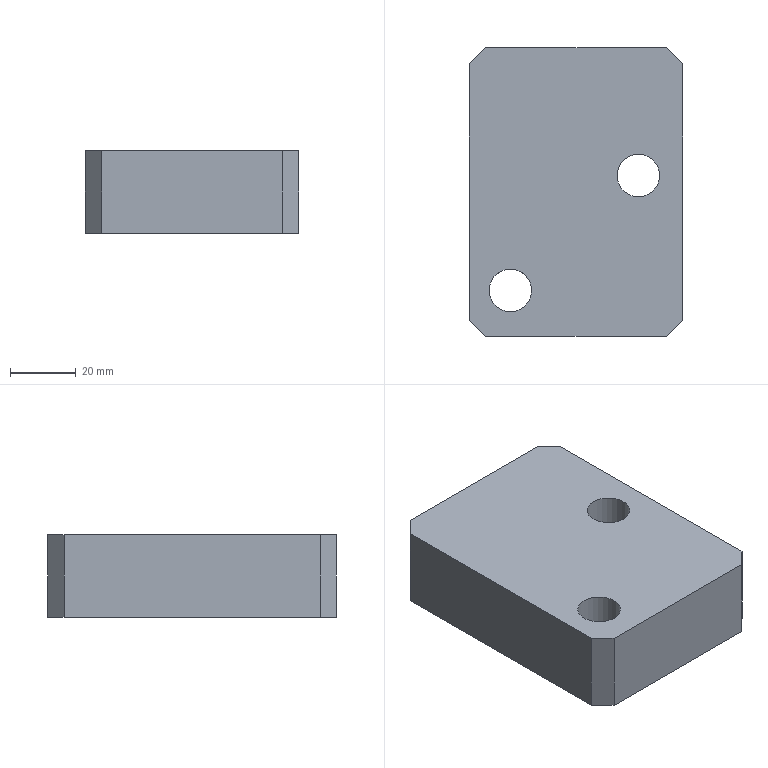Part | STEP file | 433_id2094_x_t | 1 solid | 16 faces | box 65 x 88 x 25 mm | volume 129688 mm3 | plane 12 | cylinder 4 | commonest cylinder face diameters 13 x2 20 x2
STEP:
#1=CARTESIAN_POINT('',(0.,0.,0.));
#2=DIRECTION('',(0.,0.,1.));
#3=DIRECTION('',(1.,0.,0.));
#4=AXIS2_PLACEMENT_3D('',#1,#2,#3);
#5=CARTESIAN_POINT('',(-51.,-323.071,3.));
#6=VERTEX_POINT('',#5);
#7=CARTESIAN_POINT('',(-51.,-245.,3.));
#8=VERTEX_POINT('',#7);
#9=CARTESIAN_POINT('',(-51.,625.206,3.));
#10=DIRECTION('',(0.,1.,0.));
#11=VECTOR('',#10,1.);
#12=LINE('',#9,#11);
#13=CARTESIAN_POINT('',(-51.,617.983,-1.));
#14=DIRECTION('',(-1.,0.,0.));
#15=DIRECTION('',(0.,0.,1.));
#16=AXIS2_PLACEMENT_3D('',#13,#14,#15);
#17=PLANE('',#16);
#18=CARTESIAN_POINT('',(4.,7.223));
#19=DIRECTION('',(0.,1.));
#20=VECTOR('',#19,1.);
#21=LINE('',#18,#20);
#22=(GEOMETRIC_REPRESENTATION_CONTEXT(2)PARAMETRIC_REPRESENTATION_CONTEXT()REPRESENTATION_CONTEXT('',''));
#23=DEFINITIONAL_REPRESENTATION('',(#21),#22);
#24=PCURVE('',#17,#23);
#25=CARTESIAN_POINT('',(-678.966,625.206,3.));
#26=DIRECTION('',(0.,0.,1.));
#27=DIRECTION('',(1.,0.,0.));
#28=AXIS2_PLACEMENT_3D('',#25,#26,#27);
#29=PLANE('',#28);
#30=CARTESIAN_POINT('',(627.966,0.));
#31=DIRECTION('',(0.,1.));
#32=VECTOR('',#31,1.);
#33=LINE('',#30,#32);
#34=(GEOMETRIC_REPRESENTATION_CONTEXT(2)PARAMETRIC_REPRESENTATION_CONTEXT()REPRESENTATION_CONTEXT('',''));
#35=DEFINITIONAL_REPRESENTATION('',(#33),#34);
#36=PCURVE('',#29,#35);
#37=SURFACE_CURVE('',#12,(#24,#36),.PCURVE_S1.);
#38=EDGE_CURVE('',#6,#8,#37,.T.);
#39=ORIENTED_EDGE('',*,*,#38,.T.);
#40=CARTESIAN_POINT('',(-51.,-245.,-22.));
#41=VERTEX_POINT('',#40);
#42=CARTESIAN_POINT('',(-51.,-245.,-17.));
#43=DIRECTION('',(0.,0.,1.));
#44=VECTOR('',#43,1.);
#45=LINE('',#42,#44);
#46=CARTESIAN_POINT('',(-16.,-862.983));
#47=DIRECTION('',(1.,0.));
#48=VECTOR('',#47,1.);
#49=LINE('',#46,#48);
#50=(GEOMETRIC_REPRESENTATION_CONTEXT(2)PARAMETRIC_REPRESENTATION_CONTEXT()REPRESENTATION_CONTEXT('',''));
#51=DEFINITIONAL_REPRESENTATION('',(#49),#50);
#52=PCURVE('',#17,#51);
#53=CARTESIAN_POINT('',(-51.,-245.,-1.));
#54=DIRECTION('',(0.7071,-0.7071,0.));
#55=DIRECTION('',(0.,0.,1.));
#56=AXIS2_PLACEMENT_3D('',#53,#54,#55);
#57=PLANE('',#56);
#58=CARTESIAN_POINT('',(-16.,0.));
#59=DIRECTION('',(1.,0.));
#60=VECTOR('',#59,1.);
#61=LINE('',#58,#60);
#62=(GEOMETRIC_REPRESENTATION_CONTEXT(2)PARAMETRIC_REPRESENTATION_CONTEXT()REPRESENTATION_CONTEXT('',''));
#63=DEFINITIONAL_REPRESENTATION('',(#61),#62);
#64=PCURVE('',#57,#63);
#65=SURFACE_CURVE('',#45,(#52,#64),.PCURVE_S1.);
#66=EDGE_CURVE('',#41,#8,#65,.T.);
#67=ORIENTED_EDGE('',*,*,#66,.F.);
#68=CARTESIAN_POINT('',(-51.,-323.071,-22.));
#69=VERTEX_POINT('',#68);
#70=CARTESIAN_POINT('',(-51.,625.206,-22.));
#71=DIRECTION('',(0.,1.,0.));
#72=VECTOR('',#71,1.);
#73=LINE('',#70,#72);
#74=CARTESIAN_POINT('',(-21.,7.223));
#75=DIRECTION('',(0.,1.));
#76=VECTOR('',#75,1.);
#77=LINE('',#74,#76);
#78=(GEOMETRIC_REPRESENTATION_CONTEXT(2)PARAMETRIC_REPRESENTATION_CONTEXT()REPRESENTATION_CONTEXT('',''));
#79=DEFINITIONAL_REPRESENTATION('',(#77),#78);
#80=PCURVE('',#17,#79);
#81=CARTESIAN_POINT('',(-678.966,625.206,-22.));
#82=DIRECTION('',(0.,0.,1.));
#83=DIRECTION('',(1.,0.,0.));
#84=AXIS2_PLACEMENT_3D('',#81,#82,#83);
#85=PLANE('',#84);
#86=CARTESIAN_POINT('',(627.966,0.));
#87=DIRECTION('',(0.,1.));
#88=VECTOR('',#87,1.);
#89=LINE('',#86,#88);
#90=(GEOMETRIC_REPRESENTATION_CONTEXT(2)PARAMETRIC_REPRESENTATION_CONTEXT()REPRESENTATION_CONTEXT('',''));
#91=DEFINITIONAL_REPRESENTATION('',(#89),#90);
#92=PCURVE('',#85,#91);
#93=SURFACE_CURVE('',#73,(#80,#92),.PCURVE_S1.);
#94=EDGE_CURVE('',#69,#41,#93,.T.);
#95=ORIENTED_EDGE('',*,*,#94,.F.);
#96=CARTESIAN_POINT('',(-51.,-323.071,-1.));
#97=DIRECTION('',(0.,0.,-1.));
#98=VECTOR('',#97,1.);
#99=LINE('',#96,#98);
#100=CARTESIAN_POINT('',(0.,-941.054));
#101=DIRECTION('',(-1.,0.));
#102=VECTOR('',#101,1.);
#103=LINE('',#100,#102);
#104=(GEOMETRIC_REPRESENTATION_CONTEXT(2)PARAMETRIC_REPRESENTATION_CONTEXT()REPRESENTATION_CONTEXT('',''));
#105=DEFINITIONAL_REPRESENTATION('',(#103),#104);
#106=PCURVE('',#17,#105);
#107=CARTESIAN_POINT('',(-47.536,-326.536,49.));
#108=DIRECTION('',(0.7071,0.7071,0.));
#109=DIRECTION('',(0.,0.,1.));
#110=AXIS2_PLACEMENT_3D('',#107,#108,#109);
#111=PLANE('',#110);
#112=CARTESIAN_POINT('',(-50.,-4.899));
#113=DIRECTION('',(-1.,0.));
#114=VECTOR('',#113,1.);
#115=LINE('',#112,#114);
#116=(GEOMETRIC_REPRESENTATION_CONTEXT(2)PARAMETRIC_REPRESENTATION_CONTEXT()REPRESENTATION_CONTEXT('',''));
#117=DEFINITIONAL_REPRESENTATION('',(#115),#116);
#118=PCURVE('',#111,#117);
#119=SURFACE_CURVE('',#99,(#106,#118),.PCURVE_S1.);
#120=EDGE_CURVE('',#6,#69,#119,.T.);
#121=ORIENTED_EDGE('',*,*,#120,.F.);
#122=EDGE_LOOP('',(#39,#67,#95,#121));
#123=FACE_BOUND('',#122,.T.);
#124=ADVANCED_FACE('',(#123),#17,.T.);
#125=CARTESIAN_POINT('',(14.,-245.,-22.));
#126=VERTEX_POINT('',#125);
#127=CARTESIAN_POINT('',(14.,-323.071,-22.));
#128=VERTEX_POINT('',#127);
#129=CARTESIAN_POINT('',(14.,625.206,-22.));
#130=DIRECTION('',(0.,-1.,0.));
#131=VECTOR('',#130,1.);
#132=LINE('',#129,#131);
#133=CARTESIAN_POINT('',(14.,617.983,-1.));
#134=DIRECTION('',(1.,0.,0.));
#135=DIRECTION('',(0.,0.,-1.));
#136=AXIS2_PLACEMENT_3D('',#133,#134,#135);
#137=PLANE('',#136);
#138=CARTESIAN_POINT('',(21.,7.223));
#139=DIRECTION('',(0.,-1.));
#140=VECTOR('',#139,1.);
#141=LINE('',#138,#140);
#142=(GEOMETRIC_REPRESENTATION_CONTEXT(2)PARAMETRIC_REPRESENTATION_CONTEXT()REPRESENTATION_CONTEXT('',''));
#143=DEFINITIONAL_REPRESENTATION('',(#141),#142);
#144=PCURVE('',#137,#143);
#145=CARTESIAN_POINT('',(692.966,0.));
#146=DIRECTION('',(0.,-1.));
#147=VECTOR('',#146,1.);
#148=LINE('',#145,#147);
#149=(GEOMETRIC_REPRESENTATION_CONTEXT(2)PARAMETRIC_REPRESENTATION_CONTEXT()REPRESENTATION_CONTEXT('',''));
#150=DEFINITIONAL_REPRESENTATION('',(#148),#149);
#151=PCURVE('',#85,#150);
#152=SURFACE_CURVE('',#132,(#144,#151),.PCURVE_S1.);
#153=EDGE_CURVE('',#126,#128,#152,.T.);
#154=ORIENTED_EDGE('',*,*,#153,.F.);
#155=CARTESIAN_POINT('',(14.,-245.,3.));
#156=VERTEX_POINT('',#155);
#157=CARTESIAN_POINT('',(14.,-245.,3.));
#158=DIRECTION('',(0.,0.,-1.));
#159=VECTOR('',#158,1.);
#160=LINE('',#157,#159);
#161=CARTESIAN_POINT('',(-4.,-862.983));
#162=DIRECTION('',(1.,0.));
#163=VECTOR('',#162,1.);
#164=LINE('',#161,#163);
#165=(GEOMETRIC_REPRESENTATION_CONTEXT(2)PARAMETRIC_REPRESENTATION_CONTEXT()REPRESENTATION_CONTEXT('',''));
#166=DEFINITIONAL_REPRESENTATION('',(#164),#165);
#167=PCURVE('',#137,#166);
#168=CARTESIAN_POINT('',(9.,-240.,4.));
#169=DIRECTION('',(-0.7071,-0.7071,0.));
#170=DIRECTION('',(0.,0.,1.));
#171=AXIS2_PLACEMENT_3D('',#168,#169,#170);
#172=PLANE('',#171);
#173=CARTESIAN_POINT('',(-1.,-7.071));
#174=DIRECTION('',(-1.,0.));
#175=VECTOR('',#174,1.);
#176=LINE('',#173,#175);
#177=(GEOMETRIC_REPRESENTATION_CONTEXT(2)PARAMETRIC_REPRESENTATION_CONTEXT()REPRESENTATION_CONTEXT('',''));
#178=DEFINITIONAL_REPRESENTATION('',(#176),#177);
#179=PCURVE('',#172,#178);
#180=SURFACE_CURVE('',#160,(#167,#179),.PCURVE_S1.);
#181=EDGE_CURVE('',#156,#126,#180,.T.);
#182=ORIENTED_EDGE('',*,*,#181,.F.);
#183=CARTESIAN_POINT('',(14.,-323.071,3.));
#184=VERTEX_POINT('',#183);
#185=CARTESIAN_POINT('',(14.,625.206,3.));
#186=DIRECTION('',(0.,-1.,0.));
#187=VECTOR('',#186,1.);
#188=LINE('',#185,#187);
#189=CARTESIAN_POINT('',(-4.,7.223));
#190=DIRECTION('',(0.,-1.));
#191=VECTOR('',#190,1.);
#192=LINE('',#189,#191);
#193=(GEOMETRIC_REPRESENTATION_CONTEXT(2)PARAMETRIC_REPRESENTATION_CONTEXT()REPRESENTATION_CONTEXT('',''));
#194=DEFINITIONAL_REPRESENTATION('',(#192),#193);
#195=PCURVE('',#137,#194);
#196=CARTESIAN_POINT('',(692.966,0.));
#197=DIRECTION('',(0.,-1.));
#198=VECTOR('',#197,1.);
#199=LINE('',#196,#198);
#200=(GEOMETRIC_REPRESENTATION_CONTEXT(2)PARAMETRIC_REPRESENTATION_CONTEXT()REPRESENTATION_CONTEXT('',''));
#201=DEFINITIONAL_REPRESENTATION('',(#199),#200);
#202=PCURVE('',#29,#201);
#203=SURFACE_CURVE('',#188,(#195,#202),.PCURVE_S1.);
#204=EDGE_CURVE('',#156,#184,#203,.T.);
#205=ORIENTED_EDGE('',*,*,#204,.T.);
#206=CARTESIAN_POINT('',(14.,-323.071,-1.));
#207=DIRECTION('',(0.,0.,1.));
#208=VECTOR('',#207,1.);
#209=LINE('',#206,#208);
#210=CARTESIAN_POINT('',(0.,-941.054));
#211=DIRECTION('',(-1.,0.));
#212=VECTOR('',#211,1.);
#213=LINE('',#210,#212);
#214=(GEOMETRIC_REPRESENTATION_CONTEXT(2)PARAMETRIC_REPRESENTATION_CONTEXT()REPRESENTATION_CONTEXT('',''));
#215=DEFINITIONAL_REPRESENTATION('',(#213),#214);
#216=PCURVE('',#137,#215);
#217=CARTESIAN_POINT('',(12.536,-324.536,-1.));
#218=DIRECTION('',(-0.7071,0.7071,0.));
#219=DIRECTION('',(0.,0.,1.));
#220=AXIS2_PLACEMENT_3D('',#217,#218,#219);
#221=PLANE('',#220);
#222=CARTESIAN_POINT('',(0.,2.071));
#223=DIRECTION('',(1.,0.));
#224=VECTOR('',#223,1.);
#225=LINE('',#222,#224);
#226=(GEOMETRIC_REPRESENTATION_CONTEXT(2)PARAMETRIC_REPRESENTATION_CONTEXT()REPRESENTATION_CONTEXT('',''));
#227=DEFINITIONAL_REPRESENTATION('',(#225),#226);
#228=PCURVE('',#221,#227);
#229=SURFACE_CURVE('',#209,(#216,#228),.PCURVE_S1.);
#230=EDGE_CURVE('',#128,#184,#229,.T.);
#231=ORIENTED_EDGE('',*,*,#230,.F.);
#232=EDGE_LOOP('',(#154,#182,#205,#231));
#233=FACE_BOUND('',#232,.T.);
#234=ADVANCED_FACE('',(#233),#137,.T.);
#235=CARTESIAN_POINT('',(-38.5,-324.,-22.));
#236=VERTEX_POINT('',#235);
#237=CARTESIAN_POINT('',(-38.5,-304.,-22.));
#238=VERTEX_POINT('',#237);
#239=CARTESIAN_POINT('',(-38.5,-314.,-22.));
#240=DIRECTION('',(0.,0.,-1.));
#241=DIRECTION('',(0.,-1.,0.));
#242=AXIS2_PLACEMENT_3D('',#239,#240,#241);
#243=CIRCLE('',#242,10.);
#244=CARTESIAN_POINT('',(640.466,-949.206));
#245=CARTESIAN_POINT('',(623.146,-949.206));
#246=CARTESIAN_POINT('',(631.806,-934.206));
#247=CARTESIAN_POINT('',(640.466,-919.206));
#248=CARTESIAN_POINT('',(649.127,-934.206));
#249=CARTESIAN_POINT('',(657.787,-949.206));
#250=CARTESIAN_POINT('',(640.466,-949.206));
#251=(BOUNDED_CURVE()B_SPLINE_CURVE(2,(#244,#245,#246,#247,#248,#249,#250),.UNSPECIFIED.,.T.,.F.)B_SPLINE_CURVE_WITH_KNOTS((1,2,2,2,2,1),(-2.094,0.,2.094,4.189,6.283,8.378),.UNSPECIFIED.)CURVE()GEOMETRIC_REPRESENTATION_ITEM()RATIONAL_B_SPLINE_CURVE((1.,0.5,1.,0.5,1.,0.5,1.))REPRESENTATION_ITEM(''));
#252=(GEOMETRIC_REPRESENTATION_CONTEXT(2)PARAMETRIC_REPRESENTATION_CONTEXT()REPRESENTATION_CONTEXT('',''));
#253=DEFINITIONAL_REPRESENTATION('',(#251),#252);
#254=PCURVE('',#85,#253);
#255=CARTESIAN_POINT('',(-38.5,-314.,3.));
#256=DIRECTION('',(0.,0.,1.));
#257=DIRECTION('',(1.,0.,0.));
#258=AXIS2_PLACEMENT_3D('',#255,#256,#257);
#259=CYLINDRICAL_SURFACE('',#258,10.);
#260=CARTESIAN_POINT('',(4.712,-25.));
#261=DIRECTION('',(-1.,0.));
#262=VECTOR('',#261,1.);
#263=LINE('',#260,#262);
#264=(GEOMETRIC_REPRESENTATION_CONTEXT(2)PARAMETRIC_REPRESENTATION_CONTEXT()REPRESENTATION_CONTEXT('',''));
#265=DEFINITIONAL_REPRESENTATION('',(#263),#264);
#266=PCURVE('',#259,#265);
#267=SURFACE_CURVE('',#243,(#254,#266),.PCURVE_S1.);
#268=EDGE_CURVE('',#236,#238,#267,.T.);
#269=ORIENTED_EDGE('',*,*,#268,.F.);
#270=CARTESIAN_POINT('',(-38.5,-314.,-22.));
#271=DIRECTION('',(0.,0.,-1.));
#272=DIRECTION('',(0.,-1.,0.));
#273=AXIS2_PLACEMENT_3D('',#270,#271,#272);
#274=CIRCLE('',#273,10.);
#275=CARTESIAN_POINT('',(640.466,-949.206));
#276=CARTESIAN_POINT('',(623.146,-949.206));
#277=CARTESIAN_POINT('',(631.806,-934.206));
#278=CARTESIAN_POINT('',(640.466,-919.206));
#279=CARTESIAN_POINT('',(649.127,-934.206));
#280=CARTESIAN_POINT('',(657.787,-949.206));
#281=CARTESIAN_POINT('',(640.466,-949.206));
#282=(BOUNDED_CURVE()B_SPLINE_CURVE(2,(#275,#276,#277,#278,#279,#280,#281),.UNSPECIFIED.,.T.,.F.)B_SPLINE_CURVE_WITH_KNOTS((1,2,2,2,2,1),(-2.094,0.,2.094,4.189,6.283,8.378),.UNSPECIFIED.)CURVE()GEOMETRIC_REPRESENTATION_ITEM()RATIONAL_B_SPLINE_CURVE((1.,0.5,1.,0.5,1.,0.5,1.))REPRESENTATION_ITEM(''));
#283=(GEOMETRIC_REPRESENTATION_CONTEXT(2)PARAMETRIC_REPRESENTATION_CONTEXT()REPRESENTATION_CONTEXT('',''));
#284=DEFINITIONAL_REPRESENTATION('',(#282),#283);
#285=PCURVE('',#85,#284);
#286=CARTESIAN_POINT('',(10.996,-25.));
#287=DIRECTION('',(-1.,0.));
#288=VECTOR('',#287,1.);
#289=LINE('',#286,#288);
#290=(GEOMETRIC_REPRESENTATION_CONTEXT(2)PARAMETRIC_REPRESENTATION_CONTEXT()REPRESENTATION_CONTEXT('',''));
#291=DEFINITIONAL_REPRESENTATION('',(#289),#290);
#292=PCURVE('',#259,#291);
#293=SURFACE_CURVE('',#274,(#285,#292),.PCURVE_S1.);
#294=EDGE_CURVE('',#238,#236,#293,.T.);
#295=ORIENTED_EDGE('',*,*,#294,.F.);
#296=EDGE_LOOP('',(#269,#295));
#297=FACE_BOUND('',#296,.T.);
#298=CARTESIAN_POINT('',(0.5,-289.,-22.));
#299=VERTEX_POINT('',#298);
#300=CARTESIAN_POINT('',(0.5,-269.,-22.));
#301=VERTEX_POINT('',#300);
#302=CARTESIAN_POINT('',(0.5,-279.,-22.));
#303=DIRECTION('',(0.,0.,1.));
#304=DIRECTION('',(0.,-1.,0.));
#305=AXIS2_PLACEMENT_3D('',#302,#303,#304);
#306=CIRCLE('',#305,10.);
#307=CARTESIAN_POINT('',(679.466,-904.206));
#308=DIRECTION('',(0.,-1.));
#309=AXIS2_PLACEMENT_2D('',#307,#308);
#310=CIRCLE('',#309,10.);
#311=(GEOMETRIC_REPRESENTATION_CONTEXT(2)PARAMETRIC_REPRESENTATION_CONTEXT()REPRESENTATION_CONTEXT('',''));
#312=DEFINITIONAL_REPRESENTATION('',(#310),#311);
#313=PCURVE('',#85,#312);
#314=CARTESIAN_POINT('',(0.5,-279.,3.));
#315=DIRECTION('',(0.,0.,1.));
#316=DIRECTION('',(1.,0.,0.));
#317=AXIS2_PLACEMENT_3D('',#314,#315,#316);
#318=CYLINDRICAL_SURFACE('',#317,10.);
#319=CARTESIAN_POINT('',(4.712,-25.));
#320=DIRECTION('',(1.,0.));
#321=VECTOR('',#320,1.);
#322=LINE('',#319,#321);
#323=(GEOMETRIC_REPRESENTATION_CONTEXT(2)PARAMETRIC_REPRESENTATION_CONTEXT()REPRESENTATION_CONTEXT('',''));
#324=DEFINITIONAL_REPRESENTATION('',(#322),#323);
#325=PCURVE('',#318,#324);
#326=SURFACE_CURVE('',#306,(#313,#325),.PCURVE_S1.);
#327=EDGE_CURVE('',#299,#301,#326,.T.);
#328=ORIENTED_EDGE('',*,*,#327,.T.);
#329=CARTESIAN_POINT('',(0.5,-279.,-22.));
#330=DIRECTION('',(0.,0.,1.));
#331=DIRECTION('',(0.,-1.,0.));
#332=AXIS2_PLACEMENT_3D('',#329,#330,#331);
#333=CIRCLE('',#332,10.);
#334=CARTESIAN_POINT('',(679.466,-904.206));
#335=DIRECTION('',(0.,-1.));
#336=AXIS2_PLACEMENT_2D('',#334,#335);
#337=CIRCLE('',#336,10.);
#338=(GEOMETRIC_REPRESENTATION_CONTEXT(2)PARAMETRIC_REPRESENTATION_CONTEXT()REPRESENTATION_CONTEXT('',''));
#339=DEFINITIONAL_REPRESENTATION('',(#337),#338);
#340=PCURVE('',#85,#339);
#341=CARTESIAN_POINT('',(-1.571,-25.));
#342=DIRECTION('',(1.,0.));
#343=VECTOR('',#342,1.);
#344=LINE('',#341,#343);
#345=(GEOMETRIC_REPRESENTATION_CONTEXT(2)PARAMETRIC_REPRESENTATION_CONTEXT()REPRESENTATION_CONTEXT('',''));
#346=DEFINITIONAL_REPRESENTATION('',(#344),#345);
#347=PCURVE('',#318,#346);
#348=SURFACE_CURVE('',#333,(#340,#347),.PCURVE_S1.);
#349=EDGE_CURVE('',#301,#299,#348,.T.);
#350=ORIENTED_EDGE('',*,*,#349,.T.);
#351=EDGE_LOOP('',(#328,#350));
#352=FACE_BOUND('',#351,.T.);
#353=CARTESIAN_POINT('',(-46.,-240.,-22.));
#354=VERTEX_POINT('',#353);
#355=CARTESIAN_POINT('',(9.,-240.,-22.));
#356=VERTEX_POINT('',#355);
#357=CARTESIAN_POINT('',(-678.966,-240.,-22.));
#358=DIRECTION('',(1.,0.,0.));
#359=VECTOR('',#358,1.);
#360=LINE('',#357,#359);
#361=CARTESIAN_POINT('',(0.,-865.206));
#362=DIRECTION('',(1.,0.));
#363=VECTOR('',#362,1.);
#364=LINE('',#361,#363);
#365=(GEOMETRIC_REPRESENTATION_CONTEXT(2)PARAMETRIC_REPRESENTATION_CONTEXT()REPRESENTATION_CONTEXT('',''));
#366=DEFINITIONAL_REPRESENTATION('',(#364),#365);
#367=PCURVE('',#85,#366);
#368=CARTESIAN_POINT('',(-677.035,-240.,4.));
#369=DIRECTION('',(0.,1.,0.));
#370=DIRECTION('',(-1.,0.,0.));
#371=AXIS2_PLACEMENT_3D('',#368,#369,#370);
#372=PLANE('',#371);
#373=CARTESIAN_POINT('',(1.931,-26.));
#374=DIRECTION('',(-1.,0.));
#375=VECTOR('',#374,1.);
#376=LINE('',#373,#375);
#377=(GEOMETRIC_REPRESENTATION_CONTEXT(2)PARAMETRIC_REPRESENTATION_CONTEXT()REPRESENTATION_CONTEXT('',''));
#378=DEFINITIONAL_REPRESENTATION('',(#376),#377);
#379=PCURVE('',#372,#378);
#380=SURFACE_CURVE('',#360,(#367,#379),.PCURVE_S1.);
#381=EDGE_CURVE('',#354,#356,#380,.T.);
#382=ORIENTED_EDGE('',*,*,#381,.T.);
#383=CARTESIAN_POINT('',(9.,-240.,-22.));
#384=DIRECTION('',(-0.7071,0.7071,0.));
#385=VECTOR('',#384,1.);
#386=LINE('',#383,#385);
#387=CARTESIAN_POINT('',(687.966,-865.206));
#388=DIRECTION('',(-0.7071,0.7071));
#389=VECTOR('',#388,1.);
#390=LINE('',#387,#389);
#391=(GEOMETRIC_REPRESENTATION_CONTEXT(2)PARAMETRIC_REPRESENTATION_CONTEXT()REPRESENTATION_CONTEXT('',''));
#392=DEFINITIONAL_REPRESENTATION('',(#390),#391);
#393=PCURVE('',#85,#392);
#394=CARTESIAN_POINT('',(-26.,0.));
#395=DIRECTION('',(0.,1.));
#396=VECTOR('',#395,1.);
#397=LINE('',#394,#396);
#398=(GEOMETRIC_REPRESENTATION_CONTEXT(2)PARAMETRIC_REPRESENTATION_CONTEXT()REPRESENTATION_CONTEXT('',''));
#399=DEFINITIONAL_REPRESENTATION('',(#397),#398);
#400=PCURVE('',#172,#399);
#401=SURFACE_CURVE('',#386,(#393,#400),.PCURVE_S1.);
#402=EDGE_CURVE('',#126,#356,#401,.T.);
#403=ORIENTED_EDGE('',*,*,#402,.F.);
#404=ORIENTED_EDGE('',*,*,#153,.T.);
#405=CARTESIAN_POINT('',(9.071,-328.,-22.));
#406=VERTEX_POINT('',#405);
#407=CARTESIAN_POINT('',(12.536,-324.536,-22.));
#408=DIRECTION('',(0.7071,0.7071,0.));
#409=VECTOR('',#408,1.);
#410=LINE('',#407,#409);
#411=CARTESIAN_POINT('',(691.502,-949.741));
#412=DIRECTION('',(0.7071,0.7071));
#413=VECTOR('',#412,1.);
#414=LINE('',#411,#413);
#415=(GEOMETRIC_REPRESENTATION_CONTEXT(2)PARAMETRIC_REPRESENTATION_CONTEXT()REPRESENTATION_CONTEXT('',''));
#416=DEFINITIONAL_REPRESENTATION('',(#414),#415);
#417=PCURVE('',#85,#416);
#418=CARTESIAN_POINT('',(-21.,0.));
#419=DIRECTION('',(0.,1.));
#420=VECTOR('',#419,1.);
#421=LINE('',#418,#420);
#422=(GEOMETRIC_REPRESENTATION_CONTEXT(2)PARAMETRIC_REPRESENTATION_CONTEXT()REPRESENTATION_CONTEXT('',''));
#423=DEFINITIONAL_REPRESENTATION('',(#421),#422);
#424=PCURVE('',#221,#423);
#425=SURFACE_CURVE('',#410,(#417,#424),.PCURVE_S1.);
#426=EDGE_CURVE('',#406,#128,#425,.T.);
#427=ORIENTED_EDGE('',*,*,#426,.F.);
#428=CARTESIAN_POINT('',(-46.071,-328.,-22.));
#429=VERTEX_POINT('',#428);
#430=CARTESIAN_POINT('',(-678.966,-328.,-22.));
#431=DIRECTION('',(-1.,0.,0.));
#432=VECTOR('',#431,1.);
#433=LINE('',#430,#432);
#434=CARTESIAN_POINT('',(0.,-953.206));
#435=DIRECTION('',(-1.,0.));
#436=VECTOR('',#435,1.);
#437=LINE('',#434,#436);
#438=(GEOMETRIC_REPRESENTATION_CONTEXT(2)PARAMETRIC_REPRESENTATION_CONTEXT()REPRESENTATION_CONTEXT('',''));
#439=DEFINITIONAL_REPRESENTATION('',(#437),#438);
#440=PCURVE('',#85,#439);
#441=CARTESIAN_POINT('',(-38.5,-328.,49.));
#442=DIRECTION('',(0.,-1.,0.));
#443=DIRECTION('',(0.,0.,1.));
#444=AXIS2_PLACEMENT_3D('',#441,#442,#443);
#445=PLANE('',#444);
#446=CARTESIAN_POINT('',(-71.,640.466));
#447=DIRECTION('',(0.,1.));
#448=VECTOR('',#447,1.);
#449=LINE('',#446,#448);
#450=(GEOMETRIC_REPRESENTATION_CONTEXT(2)PARAMETRIC_REPRESENTATION_CONTEXT()REPRESENTATION_CONTEXT('',''));
#451=DEFINITIONAL_REPRESENTATION('',(#449),#450);
#452=PCURVE('',#445,#451);
#453=SURFACE_CURVE('',#433,(#440,#452),.PCURVE_S1.);
#454=EDGE_CURVE('',#406,#429,#453,.T.);
#455=ORIENTED_EDGE('',*,*,#454,.T.);
#456=CARTESIAN_POINT('',(-47.536,-326.536,-22.));
#457=DIRECTION('',(0.7071,-0.7071,0.));
#458=VECTOR('',#457,1.);
#459=LINE('',#456,#458);
#460=CARTESIAN_POINT('',(631.431,-951.741));
#461=DIRECTION('',(0.7071,-0.7071));
#462=VECTOR('',#461,1.);
#463=LINE('',#460,#462);
#464=(GEOMETRIC_REPRESENTATION_CONTEXT(2)PARAMETRIC_REPRESENTATION_CONTEXT()REPRESENTATION_CONTEXT('',''));
#465=DEFINITIONAL_REPRESENTATION('',(#463),#464);
#466=PCURVE('',#85,#465);
#467=CARTESIAN_POINT('',(-71.,0.));
#468=DIRECTION('',(0.,1.));
#469=VECTOR('',#468,1.);
#470=LINE('',#467,#469);
#471=(GEOMETRIC_REPRESENTATION_CONTEXT(2)PARAMETRIC_REPRESENTATION_CONTEXT()REPRESENTATION_CONTEXT('',''));
#472=DEFINITIONAL_REPRESENTATION('',(#470),#471);
#473=PCURVE('',#111,#472);
#474=SURFACE_CURVE('',#459,(#466,#473),.PCURVE_S1.);
#475=EDGE_CURVE('',#69,#429,#474,.T.);
#476=ORIENTED_EDGE('',*,*,#475,.F.);
#477=ORIENTED_EDGE('',*,*,#94,.T.);
#478=CARTESIAN_POINT('',(-51.,-245.,-22.));
#479=DIRECTION('',(-0.7071,-0.7071,0.));
#480=VECTOR('',#479,1.);
#481=LINE('',#478,#480);
#482=CARTESIAN_POINT('',(627.966,-870.206));
#483=DIRECTION('',(-0.7071,-0.7071));
#484=VECTOR('',#483,1.);
#485=LINE('',#482,#484);
#486=(GEOMETRIC_REPRESENTATION_CONTEXT(2)PARAMETRIC_REPRESENTATION_CONTEXT()REPRESENTATION_CONTEXT('',''));
#487=DEFINITIONAL_REPRESENTATION('',(#485),#486);
#488=PCURVE('',#85,#487);
#489=CARTESIAN_POINT('',(-21.,0.));
#490=DIRECTION('',(0.,1.));
#491=VECTOR('',#490,1.);
#492=LINE('',#489,#491);
#493=(GEOMETRIC_REPRESENTATION_CONTEXT(2)PARAMETRIC_REPRESENTATION_CONTEXT()REPRESENTATION_CONTEXT('',''));
#494=DEFINITIONAL_REPRESENTATION('',(#492),#493);
#495=PCURVE('',#57,#494);
#496=SURFACE_CURVE('',#481,(#488,#495),.PCURVE_S1.);
#497=EDGE_CURVE('',#354,#41,#496,.T.);
#498=ORIENTED_EDGE('',*,*,#497,.F.);
#499=EDGE_LOOP('',(#382,#403,#404,#427,#455,#476,#477,#498));
#500=FACE_BOUND('',#499,.T.);
#501=ADVANCED_FACE('',(#297,#352,#500),#85,.F.);
#502=CARTESIAN_POINT('',(0.5,-285.5,3.));
#503=VERTEX_POINT('',#502);
#504=CARTESIAN_POINT('',(0.5,-279.,3.));
#505=DIRECTION('',(0.,0.,-1.));
#506=DIRECTION('',(0.,-1.,0.));
#507=AXIS2_PLACEMENT_3D('',#504,#505,#506);
#508=CIRCLE('',#507,6.5);
#509=CARTESIAN_POINT('',(679.466,-910.706));
#510=CARTESIAN_POINT('',(668.208,-910.706));
#511=CARTESIAN_POINT('',(673.837,-900.956));
#512=CARTESIAN_POINT('',(679.466,-891.206));
#513=CARTESIAN_POINT('',(685.096,-900.956));
#514=CARTESIAN_POINT('',(690.725,-910.706));
#515=CARTESIAN_POINT('',(679.466,-910.706));
#516=(BOUNDED_CURVE()B_SPLINE_CURVE(2,(#509,#510,#511,#512,#513,#514,#515),.UNSPECIFIED.,.T.,.F.)B_SPLINE_CURVE_WITH_KNOTS((1,2,2,2,2,1),(-2.094,0.,2.094,4.189,6.283,8.378),.UNSPECIFIED.)CURVE()GEOMETRIC_REPRESENTATION_ITEM()RATIONAL_B_SPLINE_CURVE((1.,0.5,1.,0.5,1.,0.5,1.))REPRESENTATION_ITEM(''));
#517=(GEOMETRIC_REPRESENTATION_CONTEXT(2)PARAMETRIC_REPRESENTATION_CONTEXT()REPRESENTATION_CONTEXT('',''));
#518=DEFINITIONAL_REPRESENTATION('',(#516),#517);
#519=PCURVE('',#29,#518);
#520=CARTESIAN_POINT('',(0.5,-279.,-84.));
#521=DIRECTION('',(0.,0.,1.));
#522=DIRECTION('',(0.,-1.,0.));
#523=AXIS2_PLACEMENT_3D('',#520,#521,#522);
#524=CYLINDRICAL_SURFACE('',#523,6.5);
#525=CARTESIAN_POINT('',(6.283,87.));
#526=DIRECTION('',(-1.,0.));
#527=VECTOR('',#526,1.);
#528=LINE('',#525,#527);
#529=(GEOMETRIC_REPRESENTATION_CONTEXT(2)PARAMETRIC_REPRESENTATION_CONTEXT()REPRESENTATION_CONTEXT('',''));
#530=DEFINITIONAL_REPRESENTATION('',(#528),#529);
#531=PCURVE('',#524,#530);
#532=SURFACE_CURVE('',#508,(#519,#531),.PCURVE_S1.);
#533=EDGE_CURVE('',#503,#503,#532,.T.);
#534=ORIENTED_EDGE('',*,*,#533,.T.);
#535=EDGE_LOOP('',(#534));
#536=FACE_BOUND('',#535,.T.);
#537=CARTESIAN_POINT('',(-38.5,-320.5,3.));
#538=VERTEX_POINT('',#537);
#539=CARTESIAN_POINT('',(-38.5,-314.,3.));
#540=DIRECTION('',(0.,0.,-1.));
#541=DIRECTION('',(0.,-1.,0.));
#542=AXIS2_PLACEMENT_3D('',#539,#540,#541);
#543=CIRCLE('',#542,6.5);
#544=CARTESIAN_POINT('',(640.466,-945.706));
#545=CARTESIAN_POINT('',(629.208,-945.706));
#546=CARTESIAN_POINT('',(634.837,-935.956));
#547=CARTESIAN_POINT('',(640.466,-926.206));
#548=CARTESIAN_POINT('',(646.096,-935.956));
#549=CARTESIAN_POINT('',(651.725,-945.706));
#550=CARTESIAN_POINT('',(640.466,-945.706));
#551=(BOUNDED_CURVE()B_SPLINE_CURVE(2,(#544,#545,#546,#547,#548,#549,#550),.UNSPECIFIED.,.T.,.F.)B_SPLINE_CURVE_WITH_KNOTS((1,2,2,2,2,1),(-2.094,0.,2.094,4.189,6.283,8.378),.UNSPECIFIED.)CURVE()GEOMETRIC_REPRESENTATION_ITEM()RATIONAL_B_SPLINE_CURVE((1.,0.5,1.,0.5,1.,0.5,1.))REPRESENTATION_ITEM(''));
#552=(GEOMETRIC_REPRESENTATION_CONTEXT(2)PARAMETRIC_REPRESENTATION_CONTEXT()REPRESENTATION_CONTEXT('',''));
#553=DEFINITIONAL_REPRESENTATION('',(#551),#552);
#554=PCURVE('',#29,#553);
#555=CARTESIAN_POINT('',(-38.5,-314.,-84.));
#556=DIRECTION('',(0.,0.,1.));
#557=DIRECTION('',(0.,-1.,0.));
#558=AXIS2_PLACEMENT_3D('',#555,#556,#557);
#559=CYLINDRICAL_SURFACE('',#558,6.5);
#560=CARTESIAN_POINT('',(6.283,87.));
#561=DIRECTION('',(-1.,0.));
#562=VECTOR('',#561,1.);
#563=LINE('',#560,#562);
#564=(GEOMETRIC_REPRESENTATION_CONTEXT(2)PARAMETRIC_REPRESENTATION_CONTEXT()REPRESENTATION_CONTEXT('',''));
#565=DEFINITIONAL_REPRESENTATION('',(#563),#564);
#566=PCURVE('',#559,#565);
#567=SURFACE_CURVE('',#543,(#554,#566),.PCURVE_S1.);
#568=EDGE_CURVE('',#538,#538,#567,.T.);
#569=ORIENTED_EDGE('',*,*,#568,.T.);
#570=EDGE_LOOP('',(#569));
#571=FACE_BOUND('',#570,.T.);
#572=ORIENTED_EDGE('',*,*,#204,.F.);
#573=CARTESIAN_POINT('',(9.,-240.,3.));
#574=VERTEX_POINT('',#573);
#575=CARTESIAN_POINT('',(-762.586,531.586,3.));
#576=DIRECTION('',(0.7071,-0.7071,0.));
#577=VECTOR('',#576,1.);
#578=LINE('',#575,#577);
#579=CARTESIAN_POINT('',(-83.62,-93.62));
#580=DIRECTION('',(0.7071,-0.7071));
#581=VECTOR('',#580,1.);
#582=LINE('',#579,#581);
#583=(GEOMETRIC_REPRESENTATION_CONTEXT(2)PARAMETRIC_REPRESENTATION_CONTEXT()REPRESENTATION_CONTEXT('',''));
#584=DEFINITIONAL_REPRESENTATION('',(#582),#583);
#585=PCURVE('',#29,#584);
#586=CARTESIAN_POINT('',(-1.,1091.187));
#587=DIRECTION('',(0.,-1.));
#588=VECTOR('',#587,1.);
#589=LINE('',#586,#588);
#590=(GEOMETRIC_REPRESENTATION_CONTEXT(2)PARAMETRIC_REPRESENTATION_CONTEXT()REPRESENTATION_CONTEXT('',''));
#591=DEFINITIONAL_REPRESENTATION('',(#589),#590);
#592=PCURVE('',#172,#591);
#593=SURFACE_CURVE('',#578,(#585,#592),.PCURVE_S1.);
#594=EDGE_CURVE('',#574,#156,#593,.T.);
#595=ORIENTED_EDGE('',*,*,#594,.F.);
#596=CARTESIAN_POINT('',(-46.,-240.,3.));
#597=VERTEX_POINT('',#596);
#598=CARTESIAN_POINT('',(-678.966,-240.,3.));
#599=DIRECTION('',(1.,0.,0.));
#600=VECTOR('',#599,1.);
#601=LINE('',#598,#600);
#602=CARTESIAN_POINT('',(0.,-865.206));
#603=DIRECTION('',(1.,0.));
#604=VECTOR('',#603,1.);
#605=LINE('',#602,#604);
#606=(GEOMETRIC_REPRESENTATION_CONTEXT(2)PARAMETRIC_REPRESENTATION_CONTEXT()REPRESENTATION_CONTEXT('',''));
#607=DEFINITIONAL_REPRESENTATION('',(#605),#606);
#608=PCURVE('',#29,#607);
#609=CARTESIAN_POINT('',(1.931,-1.));
#610=DIRECTION('',(-1.,0.));
#611=VECTOR('',#610,1.);
#612=LINE('',#609,#611);
#613=(GEOMETRIC_REPRESENTATION_CONTEXT(2)PARAMETRIC_REPRESENTATION_CONTEXT()REPRESENTATION_CONTEXT('',''));
#614=DEFINITIONAL_REPRESENTATION('',(#612),#613);
#615=PCURVE('',#372,#614);
#616=SURFACE_CURVE('',#601,(#608,#615),.PCURVE_S1.);
#617=EDGE_CURVE('',#597,#574,#616,.T.);
#618=ORIENTED_EDGE('',*,*,#617,.F.);
#619=CARTESIAN_POINT('',(85.12,-108.88,3.));
#620=DIRECTION('',(0.7071,0.7071,0.));
#621=VECTOR('',#620,1.);
#622=LINE('',#619,#621);
#623=CARTESIAN_POINT('',(764.086,-734.086));
#624=DIRECTION('',(0.7071,0.7071));
#625=VECTOR('',#624,1.);
#626=LINE('',#623,#625);
#627=(GEOMETRIC_REPRESENTATION_CONTEXT(2)PARAMETRIC_REPRESENTATION_CONTEXT()REPRESENTATION_CONTEXT('',''));
#628=DEFINITIONAL_REPRESENTATION('',(#626),#627);
#629=PCURVE('',#29,#628);
#630=CARTESIAN_POINT('',(4.,-192.502));
#631=DIRECTION('',(0.,-1.));
#632=VECTOR('',#631,1.);
#633=LINE('',#630,#632);
#634=(GEOMETRIC_REPRESENTATION_CONTEXT(2)PARAMETRIC_REPRESENTATION_CONTEXT()REPRESENTATION_CONTEXT('',''));
#635=DEFINITIONAL_REPRESENTATION('',(#633),#634);
#636=PCURVE('',#57,#635);
#637=SURFACE_CURVE('',#622,(#629,#636),.PCURVE_S1.);
#638=EDGE_CURVE('',#8,#597,#637,.T.);
#639=ORIENTED_EDGE('',*,*,#638,.F.);
#640=ORIENTED_EDGE('',*,*,#38,.F.);
#641=CARTESIAN_POINT('',(-46.071,-328.,3.));
#642=VERTEX_POINT('',#641);
#643=CARTESIAN_POINT('',(-822.621,448.55,3.));
#644=DIRECTION('',(-0.7071,0.7071,0.));
#645=VECTOR('',#644,1.);
#646=LINE('',#643,#645);
#647=CARTESIAN_POINT('',(-143.655,-176.655));
#648=DIRECTION('',(-0.7071,0.7071));
#649=VECTOR('',#648,1.);
#650=LINE('',#647,#649);
#651=(GEOMETRIC_REPRESENTATION_CONTEXT(2)PARAMETRIC_REPRESENTATION_CONTEXT()REPRESENTATION_CONTEXT('',''));
#652=DEFINITIONAL_REPRESENTATION('',(#650),#651);
#653=PCURVE('',#29,#652);
#654=CARTESIAN_POINT('',(-46.,-1096.137));
#655=DIRECTION('',(0.,-1.));
#656=VECTOR('',#655,1.);
#657=LINE('',#654,#656);
#658=(GEOMETRIC_REPRESENTATION_CONTEXT(2)PARAMETRIC_REPRESENTATION_CONTEXT()REPRESENTATION_CONTEXT('',''));
#659=DEFINITIONAL_REPRESENTATION('',(#657),#658);
#660=PCURVE('',#111,#659);
#661=SURFACE_CURVE('',#646,(#653,#660),.PCURVE_S1.);
#662=EDGE_CURVE('',#642,#6,#661,.T.);
#663=ORIENTED_EDGE('',*,*,#662,.F.);
#664=CARTESIAN_POINT('',(9.071,-328.,3.));
#665=VERTEX_POINT('',#664);
#666=CARTESIAN_POINT('',(-678.966,-328.,3.));
#667=DIRECTION('',(-1.,0.,0.));
#668=VECTOR('',#667,1.);
#669=LINE('',#666,#668);
#670=CARTESIAN_POINT('',(0.,-953.206));
#671=DIRECTION('',(-1.,0.));
#672=VECTOR('',#671,1.);
#673=LINE('',#670,#672);
#674=(GEOMETRIC_REPRESENTATION_CONTEXT(2)PARAMETRIC_REPRESENTATION_CONTEXT()REPRESENTATION_CONTEXT('',''));
#675=DEFINITIONAL_REPRESENTATION('',(#673),#674);
#676=PCURVE('',#29,#675);
#677=CARTESIAN_POINT('',(-46.,640.466));
#678=DIRECTION('',(0.,1.));
#679=VECTOR('',#678,1.);
#680=LINE('',#677,#679);
#681=(GEOMETRIC_REPRESENTATION_CONTEXT(2)PARAMETRIC_REPRESENTATION_CONTEXT()REPRESENTATION_CONTEXT('',''));
#682=DEFINITIONAL_REPRESENTATION('',(#680),#681);
#683=PCURVE('',#445,#682);
#684=SURFACE_CURVE('',#669,(#676,#683),.PCURVE_S1.);
#685=EDGE_CURVE('',#665,#642,#684,.T.);
#686=ORIENTED_EDGE('',*,*,#685,.F.);
#687=CARTESIAN_POINT('',(145.155,-191.916,3.));
#688=DIRECTION('',(-0.7071,-0.7071,0.));
#689=VECTOR('',#688,1.);
#690=LINE('',#687,#689);
#691=CARTESIAN_POINT('',(824.121,-817.121));
#692=DIRECTION('',(-0.7071,-0.7071));
#693=VECTOR('',#692,1.);
#694=LINE('',#691,#693);
#695=(GEOMETRIC_REPRESENTATION_CONTEXT(2)PARAMETRIC_REPRESENTATION_CONTEXT()REPRESENTATION_CONTEXT('',''));
#696=DEFINITIONAL_REPRESENTATION('',(#694),#695);
#697=PCURVE('',#29,#696);
#698=CARTESIAN_POINT('',(4.,187.552));
#699=DIRECTION('',(0.,-1.));
#700=VECTOR('',#699,1.);
#701=LINE('',#698,#700);
#702=(GEOMETRIC_REPRESENTATION_CONTEXT(2)PARAMETRIC_REPRESENTATION_CONTEXT()REPRESENTATION_CONTEXT('',''));
#703=DEFINITIONAL_REPRESENTATION('',(#701),#702);
#704=PCURVE('',#221,#703);
#705=SURFACE_CURVE('',#690,(#697,#704),.PCURVE_S1.);
#706=EDGE_CURVE('',#184,#665,#705,.T.);
#707=ORIENTED_EDGE('',*,*,#706,.F.);
#708=EDGE_LOOP('',(#572,#595,#618,#639,#640,#663,#686,#707));
#709=FACE_BOUND('',#708,.T.);
#710=ADVANCED_FACE('',(#536,#571,#709),#29,.T.);
#711=CARTESIAN_POINT('',(0.5,-269.,-7.));
#712=VERTEX_POINT('',#711);
#713=CARTESIAN_POINT('',(0.5,-279.,-7.));
#714=DIRECTION('',(0.,0.,1.));
#715=DIRECTION('',(0.,1.,0.));
#716=AXIS2_PLACEMENT_3D('',#713,#714,#715);
#717=CIRCLE('',#716,10.);
#718=CARTESIAN_POINT('',(0.5,-279.,-7.));
#719=DIRECTION('',(0.,0.,-1.));
#720=DIRECTION('',(0.,1.,0.));
#721=AXIS2_PLACEMENT_3D('',#718,#719,#720);
#722=PLANE('',#721);
#723=CARTESIAN_POINT('',(10.,0.));
#724=CARTESIAN_POINT('',(10.,-17.321));
#725=CARTESIAN_POINT('',(-5.,-8.66));
#726=CARTESIAN_POINT('',(-20.,0.));
#727=CARTESIAN_POINT('',(-5.,8.66));
#728=CARTESIAN_POINT('',(10.,17.321));
#729=CARTESIAN_POINT('',(10.,0.));
#730=(BOUNDED_CURVE()B_SPLINE_CURVE(2,(#723,#724,#725,#726,#727,#728,#729),.UNSPECIFIED.,.T.,.F.)B_SPLINE_CURVE_WITH_KNOTS((1,2,2,2,2,1),(-2.094,0.,2.094,4.189,6.283,8.378),.UNSPECIFIED.)CURVE()GEOMETRIC_REPRESENTATION_ITEM()RATIONAL_B_SPLINE_CURVE((1.,0.5,1.,0.5,1.,0.5,1.))REPRESENTATION_ITEM(''));
#731=(GEOMETRIC_REPRESENTATION_CONTEXT(2)PARAMETRIC_REPRESENTATION_CONTEXT()REPRESENTATION_CONTEXT('',''));
#732=DEFINITIONAL_REPRESENTATION('',(#730),#731);
#733=PCURVE('',#722,#732);
#734=CARTESIAN_POINT('',(1.571,-10.));
#735=DIRECTION('',(1.,0.));
#736=VECTOR('',#735,1.);
#737=LINE('',#734,#736);
#738=(GEOMETRIC_REPRESENTATION_CONTEXT(2)PARAMETRIC_REPRESENTATION_CONTEXT()REPRESENTATION_CONTEXT('',''));
#739=DEFINITIONAL_REPRESENTATION('',(#737),#738);
#740=PCURVE('',#318,#739);
#741=SURFACE_CURVE('',#717,(#733,#740),.PCURVE_S1.);
#742=EDGE_CURVE('',#712,#712,#741,.T.);
#743=ORIENTED_EDGE('',*,*,#742,.F.);
#744=EDGE_LOOP('',(#743));
#745=FACE_BOUND('',#744,.T.);
#746=CARTESIAN_POINT('',(0.5,-272.5,-7.));
#747=VERTEX_POINT('',#746);
#748=CARTESIAN_POINT('',(0.5,-285.5,-7.));
#749=VERTEX_POINT('',#748);
#750=CARTESIAN_POINT('',(0.5,-279.,-7.));
#751=DIRECTION('',(0.,0.,-1.));
#752=DIRECTION('',(0.,1.,0.));
#753=AXIS2_PLACEMENT_3D('',#750,#751,#752);
#754=CIRCLE('',#753,6.5);
#755=CARTESIAN_POINT('',(0.,0.));
#756=DIRECTION('',(1.,0.));
#757=AXIS2_PLACEMENT_2D('',#755,#756);
#758=CIRCLE('',#757,6.5);
#759=(GEOMETRIC_REPRESENTATION_CONTEXT(2)PARAMETRIC_REPRESENTATION_CONTEXT()REPRESENTATION_CONTEXT('',''));
#760=DEFINITIONAL_REPRESENTATION('',(#758),#759);
#761=PCURVE('',#722,#760);
#762=CARTESIAN_POINT('',(3.142,77.));
#763=DIRECTION('',(-1.,0.));
#764=VECTOR('',#763,1.);
#765=LINE('',#762,#764);
#766=(GEOMETRIC_REPRESENTATION_CONTEXT(2)PARAMETRIC_REPRESENTATION_CONTEXT()REPRESENTATION_CONTEXT('',''));
#767=DEFINITIONAL_REPRESENTATION('',(#765),#766);
#768=PCURVE('',#524,#767);
#769=SURFACE_CURVE('',#754,(#761,#768),.PCURVE_S1.);
#770=EDGE_CURVE('',#747,#749,#769,.T.);
#771=ORIENTED_EDGE('',*,*,#770,.F.);
#772=CARTESIAN_POINT('',(0.5,-279.,-7.));
#773=DIRECTION('',(0.,0.,-1.));
#774=DIRECTION('',(0.,1.,0.));
#775=AXIS2_PLACEMENT_3D('',#772,#773,#774);
#776=CIRCLE('',#775,6.5);
#777=CARTESIAN_POINT('',(0.,0.));
#778=DIRECTION('',(1.,0.));
#779=AXIS2_PLACEMENT_2D('',#777,#778);
#780=CIRCLE('',#779,6.5);
#781=(GEOMETRIC_REPRESENTATION_CONTEXT(2)PARAMETRIC_REPRESENTATION_CONTEXT()REPRESENTATION_CONTEXT('',''));
#782=DEFINITIONAL_REPRESENTATION('',(#780),#781);
#783=PCURVE('',#722,#782);
#784=CARTESIAN_POINT('',(9.425,77.));
#785=DIRECTION('',(-1.,0.));
#786=VECTOR('',#785,1.);
#787=LINE('',#784,#786);
#788=(GEOMETRIC_REPRESENTATION_CONTEXT(2)PARAMETRIC_REPRESENTATION_CONTEXT()REPRESENTATION_CONTEXT('',''));
#789=DEFINITIONAL_REPRESENTATION('',(#787),#788);
#790=PCURVE('',#524,#789);
#791=SURFACE_CURVE('',#776,(#783,#790),.PCURVE_S1.);
#792=EDGE_CURVE('',#749,#747,#791,.T.);
#793=ORIENTED_EDGE('',*,*,#792,.F.);
#794=EDGE_LOOP('',(#771,#793));
#795=FACE_BOUND('',#794,.T.);
#796=ADVANCED_FACE('',(#745,#795),#722,.T.);
#797=ORIENTED_EDGE('',*,*,#742,.F.);
#798=CARTESIAN_POINT('',(0.5,-269.,-22.));
#799=CARTESIAN_POINT('',(0.5,-269.,-7.));
#800=B_SPLINE_CURVE_WITH_KNOTS('',1,(#798,#799),.UNSPECIFIED.,.F.,.F.,(2,2),(-25.,-10.),.PIECEWISE_BEZIER_KNOTS.);
#801=CARTESIAN_POINT('',(1.571,0.));
#802=DIRECTION('',(0.,1.));
#803=VECTOR('',#802,1.);
#804=LINE('',#801,#803);
#805=(GEOMETRIC_REPRESENTATION_CONTEXT(2)PARAMETRIC_REPRESENTATION_CONTEXT()REPRESENTATION_CONTEXT('',''));
#806=DEFINITIONAL_REPRESENTATION('',(#804),#805);
#807=PCURVE('',#318,#806);
#808=CARTESIAN_POINT('',(7.854,0.));
#809=DIRECTION('',(0.,1.));
#810=VECTOR('',#809,1.);
#811=LINE('',#808,#810);
#812=(GEOMETRIC_REPRESENTATION_CONTEXT(2)PARAMETRIC_REPRESENTATION_CONTEXT()REPRESENTATION_CONTEXT('',''));
#813=DEFINITIONAL_REPRESENTATION('',(#811),#812);
#814=PCURVE('',#318,#813);
#815=SEAM_CURVE('',#800,(#807,#814),.PCURVE_S1.);
#816=EDGE_CURVE('',#301,#712,#815,.T.);
#817=ORIENTED_EDGE('',*,*,#816,.F.);
#818=ORIENTED_EDGE('',*,*,#349,.T.);
#819=ORIENTED_EDGE('',*,*,#327,.T.);
#820=ORIENTED_EDGE('',*,*,#816,.T.);
#821=EDGE_LOOP('',(#797,#817,#818,#819,#820));
#822=FACE_BOUND('',#821,.F.);
#823=ADVANCED_FACE('',(#822),#318,.F.);
#824=ORIENTED_EDGE('',*,*,#533,.T.);
#825=CARTESIAN_POINT('',(0.5,-285.5,-7.));
#826=CARTESIAN_POINT('',(0.5,-285.5,3.));
#827=B_SPLINE_CURVE_WITH_KNOTS('',1,(#825,#826),.UNSPECIFIED.,.F.,.F.,(2,2),(77.,87.),.PIECEWISE_BEZIER_KNOTS.);
#828=CARTESIAN_POINT('',(0.,0.));
#829=DIRECTION('',(0.,1.));
#830=VECTOR('',#829,1.);
#831=LINE('',#828,#830);
#832=(GEOMETRIC_REPRESENTATION_CONTEXT(2)PARAMETRIC_REPRESENTATION_CONTEXT()REPRESENTATION_CONTEXT('',''));
#833=DEFINITIONAL_REPRESENTATION('',(#831),#832);
#834=PCURVE('',#524,#833);
#835=CARTESIAN_POINT('',(6.283,0.));
#836=DIRECTION('',(0.,1.));
#837=VECTOR('',#836,1.);
#838=LINE('',#835,#837);
#839=(GEOMETRIC_REPRESENTATION_CONTEXT(2)PARAMETRIC_REPRESENTATION_CONTEXT()REPRESENTATION_CONTEXT('',''));
#840=DEFINITIONAL_REPRESENTATION('',(#838),#839);
#841=PCURVE('',#524,#840);
#842=SEAM_CURVE('',#827,(#834,#841),.PCURVE_S1.);
#843=EDGE_CURVE('',#749,#503,#842,.T.);
#844=ORIENTED_EDGE('',*,*,#843,.F.);
#845=ORIENTED_EDGE('',*,*,#770,.F.);
#846=ORIENTED_EDGE('',*,*,#792,.F.);
#847=ORIENTED_EDGE('',*,*,#843,.T.);
#848=EDGE_LOOP('',(#824,#844,#845,#846,#847));
#849=FACE_BOUND('',#848,.F.);
#850=ADVANCED_FACE('',(#849),#524,.F.);
#851=CARTESIAN_POINT('',(-38.5,-304.,-7.));
#852=VERTEX_POINT('',#851);
#853=CARTESIAN_POINT('',(-38.5,-314.,-7.));
#854=DIRECTION('',(0.,0.,1.));
#855=DIRECTION('',(0.,1.,0.));
#856=AXIS2_PLACEMENT_3D('',#853,#854,#855);
#857=CIRCLE('',#856,10.);
#858=CARTESIAN_POINT('',(-38.5,-314.,-7.));
#859=DIRECTION('',(0.,0.,-1.));
#860=DIRECTION('',(0.,1.,0.));
#861=AXIS2_PLACEMENT_3D('',#858,#859,#860);
#862=PLANE('',#861);
#863=CARTESIAN_POINT('',(10.,0.));
#864=CARTESIAN_POINT('',(10.,-17.321));
#865=CARTESIAN_POINT('',(-5.,-8.66));
#866=CARTESIAN_POINT('',(-20.,0.));
#867=CARTESIAN_POINT('',(-5.,8.66));
#868=CARTESIAN_POINT('',(10.,17.321));
#869=CARTESIAN_POINT('',(10.,0.));
#870=(BOUNDED_CURVE()B_SPLINE_CURVE(2,(#863,#864,#865,#866,#867,#868,#869),.UNSPECIFIED.,.T.,.F.)B_SPLINE_CURVE_WITH_KNOTS((1,2,2,2,2,1),(-2.094,0.,2.094,4.189,6.283,8.378),.UNSPECIFIED.)CURVE()GEOMETRIC_REPRESENTATION_ITEM()RATIONAL_B_SPLINE_CURVE((1.,0.5,1.,0.5,1.,0.5,1.))REPRESENTATION_ITEM(''));
#871=(GEOMETRIC_REPRESENTATION_CONTEXT(2)PARAMETRIC_REPRESENTATION_CONTEXT()REPRESENTATION_CONTEXT('',''));
#872=DEFINITIONAL_REPRESENTATION('',(#870),#871);
#873=PCURVE('',#862,#872);
#874=CARTESIAN_POINT('',(1.571,-10.));
#875=DIRECTION('',(1.,0.));
#876=VECTOR('',#875,1.);
#877=LINE('',#874,#876);
#878=(GEOMETRIC_REPRESENTATION_CONTEXT(2)PARAMETRIC_REPRESENTATION_CONTEXT()REPRESENTATION_CONTEXT('',''));
#879=DEFINITIONAL_REPRESENTATION('',(#877),#878);
#880=PCURVE('',#259,#879);
#881=SURFACE_CURVE('',#857,(#873,#880),.PCURVE_S1.);
#882=EDGE_CURVE('',#852,#852,#881,.T.);
#883=ORIENTED_EDGE('',*,*,#882,.F.);
#884=EDGE_LOOP('',(#883));
#885=FACE_BOUND('',#884,.T.);
#886=CARTESIAN_POINT('',(-38.5,-307.5,-7.));
#887=VERTEX_POINT('',#886);
#888=CARTESIAN_POINT('',(-38.5,-320.5,-7.));
#889=VERTEX_POINT('',#888);
#890=CARTESIAN_POINT('',(-38.5,-314.,-7.));
#891=DIRECTION('',(0.,0.,-1.));
#892=DIRECTION('',(0.,1.,0.));
#893=AXIS2_PLACEMENT_3D('',#890,#891,#892);
#894=CIRCLE('',#893,6.5);
#895=CARTESIAN_POINT('',(0.,0.));
#896=DIRECTION('',(1.,0.));
#897=AXIS2_PLACEMENT_2D('',#895,#896);
#898=CIRCLE('',#897,6.5);
#899=(GEOMETRIC_REPRESENTATION_CONTEXT(2)PARAMETRIC_REPRESENTATION_CONTEXT()REPRESENTATION_CONTEXT('',''));
#900=DEFINITIONAL_REPRESENTATION('',(#898),#899);
#901=PCURVE('',#862,#900);
#902=CARTESIAN_POINT('',(3.142,77.));
#903=DIRECTION('',(-1.,0.));
#904=VECTOR('',#903,1.);
#905=LINE('',#902,#904);
#906=(GEOMETRIC_REPRESENTATION_CONTEXT(2)PARAMETRIC_REPRESENTATION_CONTEXT()REPRESENTATION_CONTEXT('',''));
#907=DEFINITIONAL_REPRESENTATION('',(#905),#906);
#908=PCURVE('',#559,#907);
#909=SURFACE_CURVE('',#894,(#901,#908),.PCURVE_S1.);
#910=EDGE_CURVE('',#887,#889,#909,.T.);
#911=ORIENTED_EDGE('',*,*,#910,.F.);
#912=CARTESIAN_POINT('',(-38.5,-314.,-7.));
#913=DIRECTION('',(0.,0.,-1.));
#914=DIRECTION('',(0.,1.,0.));
#915=AXIS2_PLACEMENT_3D('',#912,#913,#914);
#916=CIRCLE('',#915,6.5);
#917=CARTESIAN_POINT('',(0.,0.));
#918=DIRECTION('',(1.,0.));
#919=AXIS2_PLACEMENT_2D('',#917,#918);
#920=CIRCLE('',#919,6.5);
#921=(GEOMETRIC_REPRESENTATION_CONTEXT(2)PARAMETRIC_REPRESENTATION_CONTEXT()REPRESENTATION_CONTEXT('',''));
#922=DEFINITIONAL_REPRESENTATION('',(#920),#921);
#923=PCURVE('',#862,#922);
#924=CARTESIAN_POINT('',(9.425,77.));
#925=DIRECTION('',(-1.,0.));
#926=VECTOR('',#925,1.);
#927=LINE('',#924,#926);
#928=(GEOMETRIC_REPRESENTATION_CONTEXT(2)PARAMETRIC_REPRESENTATION_CONTEXT()REPRESENTATION_CONTEXT('',''));
#929=DEFINITIONAL_REPRESENTATION('',(#927),#928);
#930=PCURVE('',#559,#929);
#931=SURFACE_CURVE('',#916,(#923,#930),.PCURVE_S1.);
#932=EDGE_CURVE('',#889,#887,#931,.T.);
#933=ORIENTED_EDGE('',*,*,#932,.F.);
#934=EDGE_LOOP('',(#911,#933));
#935=FACE_BOUND('',#934,.T.);
#936=ADVANCED_FACE('',(#885,#935),#862,.T.);
#937=ORIENTED_EDGE('',*,*,#568,.T.);
#938=CARTESIAN_POINT('',(-38.5,-320.5,-7.));
#939=CARTESIAN_POINT('',(-38.5,-320.5,3.));
#940=B_SPLINE_CURVE_WITH_KNOTS('',1,(#938,#939),.UNSPECIFIED.,.F.,.F.,(2,2),(77.,87.),.PIECEWISE_BEZIER_KNOTS.);
#941=CARTESIAN_POINT('',(0.,0.));
#942=DIRECTION('',(0.,1.));
#943=VECTOR('',#942,1.);
#944=LINE('',#941,#943);
#945=(GEOMETRIC_REPRESENTATION_CONTEXT(2)PARAMETRIC_REPRESENTATION_CONTEXT()REPRESENTATION_CONTEXT('',''));
#946=DEFINITIONAL_REPRESENTATION('',(#944),#945);
#947=PCURVE('',#559,#946);
#948=CARTESIAN_POINT('',(6.283,0.));
#949=DIRECTION('',(0.,1.));
#950=VECTOR('',#949,1.);
#951=LINE('',#948,#950);
#952=(GEOMETRIC_REPRESENTATION_CONTEXT(2)PARAMETRIC_REPRESENTATION_CONTEXT()REPRESENTATION_CONTEXT('',''));
#953=DEFINITIONAL_REPRESENTATION('',(#951),#952);
#954=PCURVE('',#559,#953);
#955=SEAM_CURVE('',#940,(#947,#954),.PCURVE_S1.);
#956=EDGE_CURVE('',#889,#538,#955,.T.);
#957=ORIENTED_EDGE('',*,*,#956,.F.);
#958=ORIENTED_EDGE('',*,*,#910,.F.);
#959=ORIENTED_EDGE('',*,*,#932,.F.);
#960=ORIENTED_EDGE('',*,*,#956,.T.);
#961=EDGE_LOOP('',(#937,#957,#958,#959,#960));
#962=FACE_BOUND('',#961,.F.);
#963=ADVANCED_FACE('',(#962),#559,.F.);
#964=ORIENTED_EDGE('',*,*,#882,.F.);
#965=CARTESIAN_POINT('',(-38.5,-304.,-22.));
#966=CARTESIAN_POINT('',(-38.5,-304.,-7.));
#967=B_SPLINE_CURVE_WITH_KNOTS('',1,(#965,#966),.UNSPECIFIED.,.F.,.F.,(2,2),(-25.,-10.),.PIECEWISE_BEZIER_KNOTS.);
#968=CARTESIAN_POINT('',(1.571,0.));
#969=DIRECTION('',(0.,1.));
#970=VECTOR('',#969,1.);
#971=LINE('',#968,#970);
#972=(GEOMETRIC_REPRESENTATION_CONTEXT(2)PARAMETRIC_REPRESENTATION_CONTEXT()REPRESENTATION_CONTEXT('',''));
#973=DEFINITIONAL_REPRESENTATION('',(#971),#972);
#974=PCURVE('',#259,#973);
#975=CARTESIAN_POINT('',(7.854,0.));
#976=DIRECTION('',(0.,1.));
#977=VECTOR('',#976,1.);
#978=LINE('',#975,#977);
#979=(GEOMETRIC_REPRESENTATION_CONTEXT(2)PARAMETRIC_REPRESENTATION_CONTEXT()REPRESENTATION_CONTEXT('',''));
#980=DEFINITIONAL_REPRESENTATION('',(#978),#979);
#981=PCURVE('',#259,#980);
#982=SEAM_CURVE('',#967,(#974,#981),.PCURVE_S1.);
#983=EDGE_CURVE('',#238,#852,#982,.T.);
#984=ORIENTED_EDGE('',*,*,#983,.F.);
#985=ORIENTED_EDGE('',*,*,#268,.F.);
#986=ORIENTED_EDGE('',*,*,#294,.F.);
#987=ORIENTED_EDGE('',*,*,#983,.T.);
#988=EDGE_LOOP('',(#964,#984,#985,#986,#987));
#989=FACE_BOUND('',#988,.F.);
#990=ADVANCED_FACE('',(#989),#259,.F.);
#991=ORIENTED_EDGE('',*,*,#685,.T.);
#992=CARTESIAN_POINT('',(-46.071,-328.,49.));
#993=DIRECTION('',(0.,0.,1.));
#994=VECTOR('',#993,1.);
#995=LINE('',#992,#994);
#996=CARTESIAN_POINT('',(0.,7.571));
#997=DIRECTION('',(1.,0.));
#998=VECTOR('',#997,1.);
#999=LINE('',#996,#998);
#1000=(GEOMETRIC_REPRESENTATION_CONTEXT(2)PARAMETRIC_REPRESENTATION_CONTEXT()REPRESENTATION_CONTEXT('',''));
#1001=DEFINITIONAL_REPRESENTATION('',(#999),#1000);
#1002=PCURVE('',#445,#1001);
#1003=CARTESIAN_POINT('',(0.,2.071));
#1004=DIRECTION('',(1.,0.));
#1005=VECTOR('',#1004,1.);
#1006=LINE('',#1003,#1005);
#1007=(GEOMETRIC_REPRESENTATION_CONTEXT(2)PARAMETRIC_REPRESENTATION_CONTEXT()REPRESENTATION_CONTEXT('',''));
#1008=DEFINITIONAL_REPRESENTATION('',(#1006),#1007);
#1009=PCURVE('',#111,#1008);
#1010=SURFACE_CURVE('',#995,(#1002,#1009),.PCURVE_S1.);
#1011=EDGE_CURVE('',#429,#642,#1010,.T.);
#1012=ORIENTED_EDGE('',*,*,#1011,.F.);
#1013=ORIENTED_EDGE('',*,*,#454,.F.);
#1014=CARTESIAN_POINT('',(9.071,-328.,49.));
#1015=DIRECTION('',(0.,0.,-1.));
#1016=VECTOR('',#1015,1.);
#1017=LINE('',#1014,#1016);
#1018=CARTESIAN_POINT('',(0.,-47.571));
#1019=DIRECTION('',(-1.,0.));
#1020=VECTOR('',#1019,1.);
#1021=LINE('',#1018,#1020);
#1022=(GEOMETRIC_REPRESENTATION_CONTEXT(2)PARAMETRIC_REPRESENTATION_CONTEXT()REPRESENTATION_CONTEXT('',''));
#1023=DEFINITIONAL_REPRESENTATION('',(#1021),#1022);
#1024=PCURVE('',#445,#1023);
#1025=CARTESIAN_POINT('',(50.,-4.899));
#1026=DIRECTION('',(-1.,0.));
#1027=VECTOR('',#1026,1.);
#1028=LINE('',#1025,#1027);
#1029=(GEOMETRIC_REPRESENTATION_CONTEXT(2)PARAMETRIC_REPRESENTATION_CONTEXT()REPRESENTATION_CONTEXT('',''));
#1030=DEFINITIONAL_REPRESENTATION('',(#1028),#1029);
#1031=PCURVE('',#221,#1030);
#1032=SURFACE_CURVE('',#1017,(#1024,#1031),.PCURVE_S1.);
#1033=EDGE_CURVE('',#665,#406,#1032,.T.);
#1034=ORIENTED_EDGE('',*,*,#1033,.F.);
#1035=EDGE_LOOP('',(#991,#1012,#1013,#1034));
#1036=FACE_BOUND('',#1035,.T.);
#1037=ADVANCED_FACE('',(#1036),#445,.T.);
#1038=ORIENTED_EDGE('',*,*,#617,.T.);
#1039=CARTESIAN_POINT('',(9.,-240.,-17.));
#1040=DIRECTION('',(0.,0.,1.));
#1041=VECTOR('',#1040,1.);
#1042=LINE('',#1039,#1041);
#1043=CARTESIAN_POINT('',(-686.035,-21.));
#1044=DIRECTION('',(0.,1.));
#1045=VECTOR('',#1044,1.);
#1046=LINE('',#1043,#1045);
#1047=(GEOMETRIC_REPRESENTATION_CONTEXT(2)PARAMETRIC_REPRESENTATION_CONTEXT()REPRESENTATION_CONTEXT('',''));
#1048=DEFINITIONAL_REPRESENTATION('',(#1046),#1047);
#1049=PCURVE('',#372,#1048);
#1050=CARTESIAN_POINT('',(-21.,0.));
#1051=DIRECTION('',(1.,0.));
#1052=VECTOR('',#1051,1.);
#1053=LINE('',#1050,#1052);
#1054=(GEOMETRIC_REPRESENTATION_CONTEXT(2)PARAMETRIC_REPRESENTATION_CONTEXT()REPRESENTATION_CONTEXT('',''));
#1055=DEFINITIONAL_REPRESENTATION('',(#1053),#1054);
#1056=PCURVE('',#172,#1055);
#1057=SURFACE_CURVE('',#1042,(#1049,#1056),.PCURVE_S1.);
#1058=EDGE_CURVE('',#356,#574,#1057,.T.);
#1059=ORIENTED_EDGE('',*,*,#1058,.F.);
#1060=ORIENTED_EDGE('',*,*,#381,.F.);
#1061=CARTESIAN_POINT('',(-46.,-240.,3.));
#1062=DIRECTION('',(0.,0.,-1.));
#1063=VECTOR('',#1062,1.);
#1064=LINE('',#1061,#1063);
#1065=CARTESIAN_POINT('',(-631.035,-1.));
#1066=DIRECTION('',(0.,-1.));
#1067=VECTOR('',#1066,1.);
#1068=LINE('',#1065,#1067);
#1069=(GEOMETRIC_REPRESENTATION_CONTEXT(2)PARAMETRIC_REPRESENTATION_CONTEXT()REPRESENTATION_CONTEXT('',''));
#1070=DEFINITIONAL_REPRESENTATION('',(#1068),#1069);
#1071=PCURVE('',#372,#1070);
#1072=CARTESIAN_POINT('',(4.,-7.071));
#1073=DIRECTION('',(-1.,0.));
#1074=VECTOR('',#1073,1.);
#1075=LINE('',#1072,#1074);
#1076=(GEOMETRIC_REPRESENTATION_CONTEXT(2)PARAMETRIC_REPRESENTATION_CONTEXT()REPRESENTATION_CONTEXT('',''));
#1077=DEFINITIONAL_REPRESENTATION('',(#1075),#1076);
#1078=PCURVE('',#57,#1077);
#1079=SURFACE_CURVE('',#1064,(#1071,#1078),.PCURVE_S1.);
#1080=EDGE_CURVE('',#597,#354,#1079,.T.);
#1081=ORIENTED_EDGE('',*,*,#1080,.F.);
#1082=EDGE_LOOP('',(#1038,#1059,#1060,#1081));
#1083=FACE_BOUND('',#1082,.T.);
#1084=ADVANCED_FACE('',(#1083),#372,.T.);
#1085=ORIENTED_EDGE('',*,*,#662,.T.);
#1086=ORIENTED_EDGE('',*,*,#120,.T.);
#1087=ORIENTED_EDGE('',*,*,#475,.T.);
#1088=ORIENTED_EDGE('',*,*,#1011,.T.);
#1089=EDGE_LOOP('',(#1085,#1086,#1087,#1088));
#1090=FACE_BOUND('',#1089,.T.);
#1091=ADVANCED_FACE('',(#1090),#111,.F.);
#1092=ORIENTED_EDGE('',*,*,#706,.T.);
#1093=ORIENTED_EDGE('',*,*,#1033,.T.);
#1094=ORIENTED_EDGE('',*,*,#426,.T.);
#1095=ORIENTED_EDGE('',*,*,#230,.T.);
#1096=EDGE_LOOP('',(#1092,#1093,#1094,#1095));
#1097=FACE_BOUND('',#1096,.T.);
#1098=ADVANCED_FACE('',(#1097),#221,.F.);
#1099=ORIENTED_EDGE('',*,*,#594,.T.);
#1100=ORIENTED_EDGE('',*,*,#181,.T.);
#1101=ORIENTED_EDGE('',*,*,#402,.T.);
#1102=ORIENTED_EDGE('',*,*,#1058,.T.);
#1103=EDGE_LOOP('',(#1099,#1100,#1101,#1102));
#1104=FACE_BOUND('',#1103,.T.);
#1105=ADVANCED_FACE('',(#1104),#172,.F.);
#1106=ORIENTED_EDGE('',*,*,#638,.T.);
#1107=ORIENTED_EDGE('',*,*,#1080,.T.);
#1108=ORIENTED_EDGE('',*,*,#497,.T.);
#1109=ORIENTED_EDGE('',*,*,#66,.T.);
#1110=EDGE_LOOP('',(#1106,#1107,#1108,#1109));
#1111=FACE_BOUND('',#1110,.T.);
#1112=ADVANCED_FACE('',(#1111),#57,.F.);
#1113=CLOSED_SHELL('',(#124,#234,#501,#710,#796,#823,#850,#936,#963,#990,#1037,#1084,#1091,#1098,#1105,#1112));
#1114=MANIFOLD_SOLID_BREP('',#1113);
#1115=(LENGTH_UNIT()NAMED_UNIT(*)SI_UNIT(.MILLI.,.METRE.));
#1116=UNCERTAINTY_MEASURE_WITH_UNIT(LENGTH_MEASURE(0.000002),#1115,'','');
#1117=(NAMED_UNIT(*)PLANE_ANGLE_UNIT()SI_UNIT($,.RADIAN.));
#1118=(NAMED_UNIT(*)SI_UNIT($,.STERADIAN.)SOLID_ANGLE_UNIT());
#1119=(GEOMETRIC_REPRESENTATION_CONTEXT(3)GLOBAL_UNCERTAINTY_ASSIGNED_CONTEXT((#1116))GLOBAL_UNIT_ASSIGNED_CONTEXT((#1115,#1117,#1118))REPRESENTATION_CONTEXT('',''));
#1120=ADVANCED_BREP_SHAPE_REPRESENTATION('',(#4,#1114),#1119);